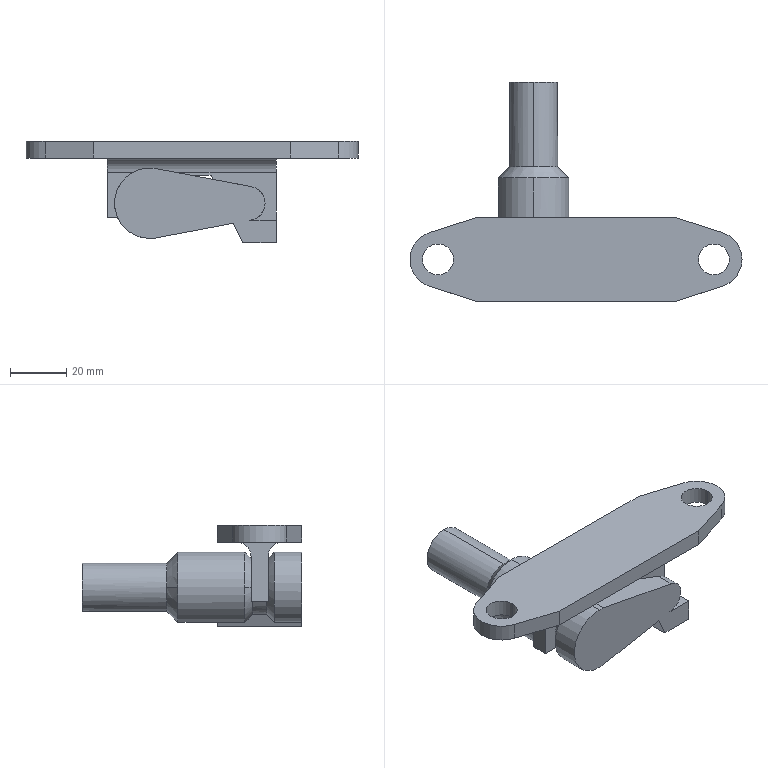Part | STEP file | 750031822 | 1 solid | 65 faces | box 118 x 78 x 36 mm | volume 64893 mm3 | plane 39 | cylinder 21 | cone 5 | commonest cylinder face diameters 25 x5 10 x4 11 x4 20 x3 12 x2 17 x2